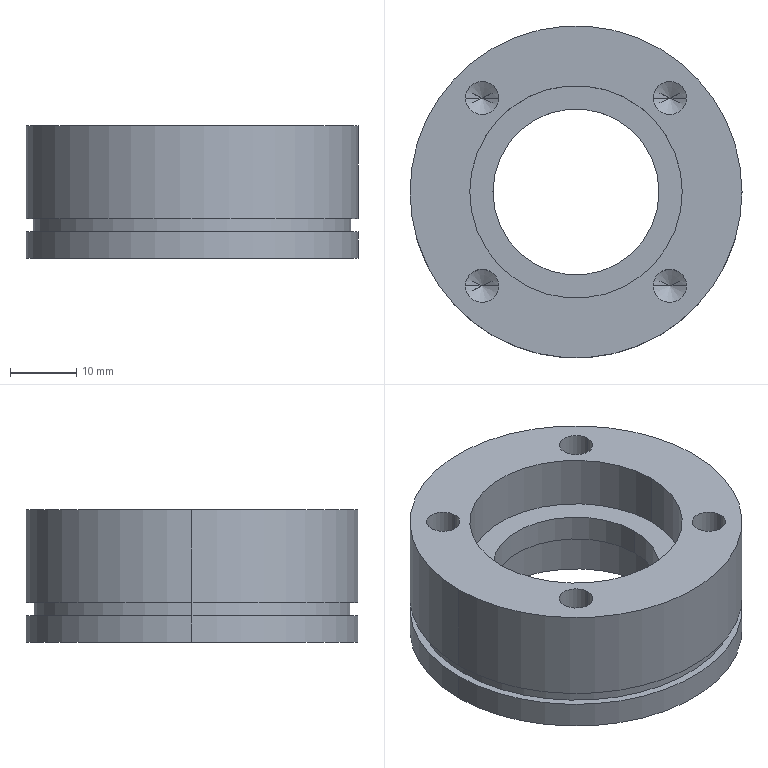Part | STEP file | Adjusting sleeve QY-1-02 | 1 solid | 42 faces | box 50 x 50 x 20 mm | volume 22863 mm3 | cylinder 24 | cone 12 | plane 6 | commonest cylinder face diameters 5 x12 32 x4 50 x4 25 x2 47.8 x2